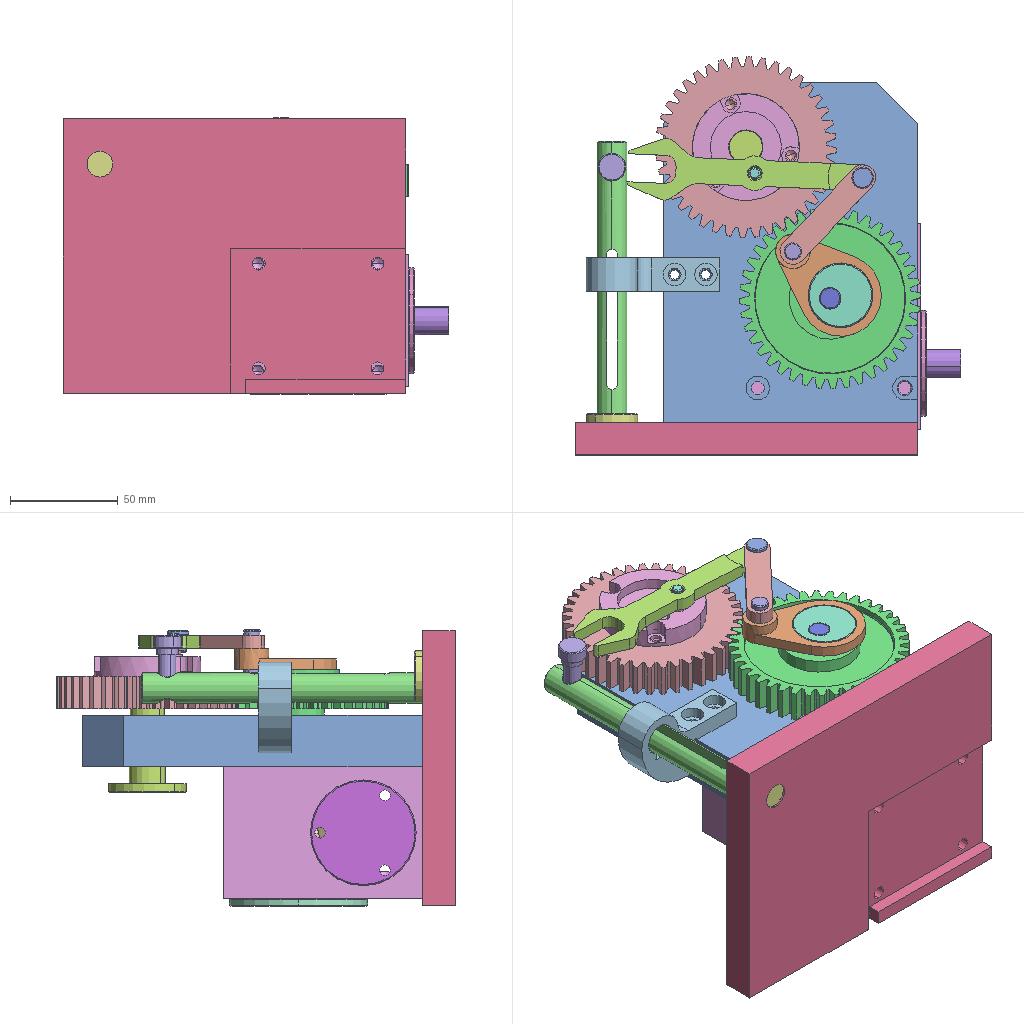Assembly | SolidWorks | 29 different items | 29 placed | box 178 x 184 x 128 mm
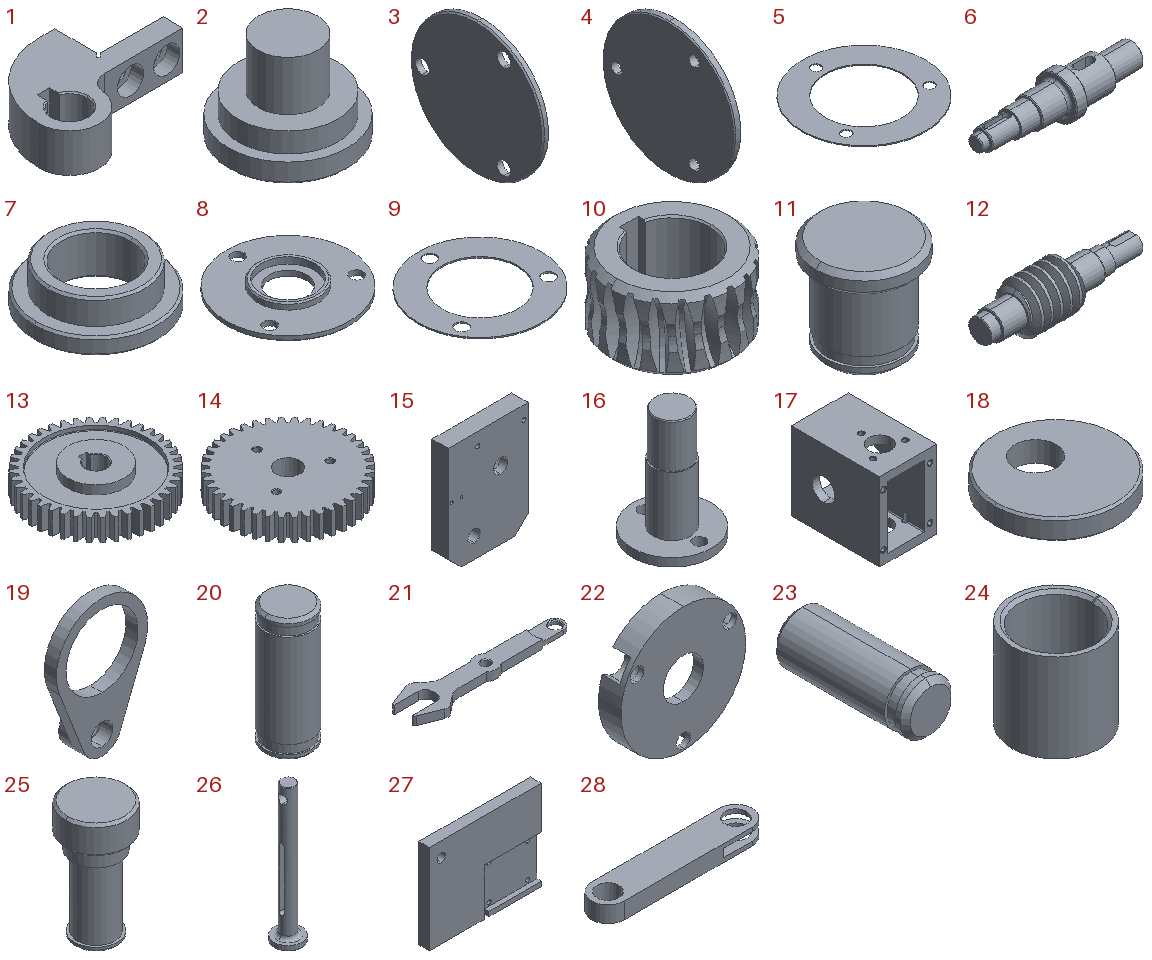Parts list (item | name | quantity | size | volume | features):
1 | - | x1 | 62 x 42 x 15.5 mm | 16029 mm3 | features ICE 3, Chamfer 1, Extrusion 1
2 | - | x1 | 24 x 24 x 18 mm | 4188 mm3 | features ICE 2, Chamfer 1, Extrusion 1
3 | - | x1 | 4.5 x 49 x 49 mm | 3890 mm3 | features ICE 3, Chamfer 1, Extrusion 1
4 | - | x1 | 6 x 64 x 64 mm | 11842 mm3 | features ICE 3, Chamfer 1, Extrusion 1
5 | - | x1 | 64 x 64 x 0.5 mm | 950.724 mm3 | features Extrusion 1, ICE 1
6 | - | x1 | 109 x 29 x 29 mm | 31302 mm3 | features ICE 8, Chamfer 1, Extrusion 1, Fillet 1
7 | - | x1 | 30 x 30 x 10 mm | 3114 mm3 | features Chamfer 2, ICE 2, Extrusion 1
8 | - | x1 | 49 x 49 x 4.5 mm | 3537 mm3 | features ICE 4, Chamfer 1, Extrusion 1
9 | - | x1 | 49 x 49 x 0.5 mm | 559.989 mm3 | features Extrusion 1, ICE 1
10 | - | x1 | 39.446 x 39.446 x 23 mm | 13124 mm3 | features Chamfer 2, CirPattern 1, Helix 1, ICE 1, Revolution 1, SweepCut 1
11 | - | x1 | 10 x 10 x 10 mm | 542.514 mm3 | features ICE 3, Chamfer 1, Extrusion 1
12 | - | x1 | 100.5 x 30 x 30 mm | 31439 mm3 | features ICE 6, Chamfer 1, Extrusion 1, Helix 1, RevCut 1, SweepCut 1
13 | - | x1 | 83.67 x 83.67 x 21 mm | 68213 mm3 | features ICE 5, Chamfer 2, CirPattern 1, Extrusion 1
14 | - | x1 | 83.602 x 83.602 x 15 mm | 71569 mm3 | features CirPattern 1, Extrusion 1, HoleWzd 1, ICE 1
15 | - | x1 | 117.5 x 24 x 160.5 mm | 414919 mm3 | features ICE 4, Chamfer 2, Extrusion 1, HoleWzd 1
16 | - | x1 | 36 x 36 x 51 mm | 14019 mm3 | features ICE 3, Chamfer 1, Extrusion 1
17 | - | x1 | 61 x 95 x 84 mm | 198920 mm3 | features HoleWzd 4, ICE 4, Extrusion 1, Fillet 1, MirrorPattern 1
18 | - | x1 | 30 x 30 x 5 mm | 3118 mm3 | features Chamfer 1, Extrusion 1, ICE 1
19 | - | x1 | 38 x 10 x 57 mm | 4565 mm3 | features ICE 3, Extrusion 1
20 | - | x1 | 8 x 8 x 21 mm | 1031 mm3 | features ICE 2, Chamfer 1, Extrusion 1, MirrorPattern 1
21 | - | x1 | 114.951 x 28.607 x 6 mm | 7418 mm3 | features ICE 2, Chamfer 1, Extrusion 1, Fillet 1, MirrorPattern 1
22 | - | x1 | 49.5 x 12 x 49.5 mm | 11403 mm3 | features ICE 6, CirPattern 1, Extrusion 1, HoleWzd 1
23 | - | x1 | 5 x 13 x 5 mm | 247.859 mm3 | features ICE 2, Chamfer 1, Extrusion 1
24 | - | x1 | 6 x 6 x 6 mm | 50.895 mm3 | features Chamfer 1, Extrusion 1, ICE 1
25 | - | x1 | 13 x 13 x 25 mm | 1836 mm3 | features ICE 4, Chamfer 1, Extrusion 1
26 | - | x1 | 28 x 28 x 140 mm | 18757 mm3 | features Chamfer 3, ICE 3, Extrusion 1, Fillet 1
27 | - | x1 | 158.5 x 15 x 127 mm | 237591 mm3 | features ICE 6, Extrusion 1, HoleWzd 1
28 | - | x1 | 59 x 12 x 6 mm | 3063 mm3 | features ICE 2, Extrusion 1
29 | angular contact ball bearings gb | x1 | - | - | -
Mates (type | each side: item.copy, entity, surface, feature):
Coincident | 27.1 plane | assembly plane | 3 times
Coincident | 27.1 face plane Cut-Extrude1 | 15.1 face plane Boss-Extrude1 | 3 times
Concentric | 14.1 face cylinder Boss-Extrude1 | 15.1 face cylinder Cut-Extrude1
Concentric | 15.1 face cylinder Cut-Extrude3 | 17.1 face cylinder Cut-Extrude3
Parallel | 15.1 face plane Boss-Extrude1 | 17.1 face plane Boss-Extrude1
Coincident | 15.1 face plane Boss-Extrude1 | 17.1 face plane Boss-Extrude1
Concentric | 13.1 face cylinder Cut-Extrude2 | 15.1 face cylinder Cut-Extrude3
Concentric | 12.1 face cylinder Boss-Extrude4 | 17.1 edge
Concentric | 10.1 face cylinder Revolve1 | 17.1 face cylinder Cut-Extrude3
Concentric | 18.1 face cylinder Boss-Extrude1 | 19.1 face cylinder Cut-Extrude1
Coincident | 18.1 face plane Boss-Extrude1 | 19.1 face plane Boss-Extrude1
Concentric | 6.1 face cylinder Boss-Extrude6 | 15.1 face cylinder Cut-Extrude1
Coincident | 6.1 face plane Cut-Extrude2 | 13.1 face plane Cut-Extrude2
Coincident | 6.1 face plane Boss-Extrude2 | 13.1 face plane Boss-Extrude3
Concentric | 6.1 face cylinder Boss-Extrude1 | 18.1 face cylinder Cut-Extrude1
Coincident | 6.1 face plane Boss-Extrude1 | 18.1 face plane Boss-Extrude1
Concentric | 15.1 face cylinder Cut-Extrude1 | 16.1 face cylinder Boss-Extrude2
Concentric | 28.1 face cylinder Cut-Extrude2 | 19.1 face cylinder Cut-Extrude1
Coincident | 28.1 face plane Boss-Extrude1 | 19.1 face plane Boss-Extrude2
Concentric | 28.1 face cylinder Cut-Extrude2 | 21.1 face cylinder Cut-Extrude2
Concentric | 11.1 face cylinder Boss-Extrude3 | 21.1 face cylinder Cut-Extrude2 | 2 times
Coincident | 28.1 face plane Boss-Extrude1 | 11.1 face plane Boss-Extrude4
Concentric | 1.1 face cylinder Cut-Extrude1 | 15.1 face cylinder M5 Tapped Hole1 | 2 times
Coincident | 1.1 face plane Boss-Extrude1 | 15.1 face plane Boss-Extrude1
Concentric | 26.1 face cylinder Boss-Extrude2 | 1.1 face cylinder Boss-Extrude1
Concentric | 25.1 face cylinder Boss-Extrude2 | 26.1 face cylinder Cut-Extrude2
Coincident | 28.1 face plane Cut-Extrude1 | 21.1 face plane Mirror1
Concentric | 19.1 face cylinder Cut-Extrude1 | 20.1 face cylinder Boss-Extrude1
Concentric | 21.1 edge | 23.1 face cylinder Boss-Extrude3
Coincident | 21.1 face plane Boss-Extrude1 | 23.1 edge
Coincident | 28.1 face plane Boss-Extrude1 | 20.1 face plane Boss-Extrude1
Concentric | 3.1 face cylinder Boss-Extrude2 | 17.1 face cylinder Mirror1
Concentric | 3.1 face cylinder Cut-Extrude2 | 17.1 face cylinder Mirror1
Coincident | 3.1 face plane Boss-Extrude1 | 17.1 face plane Boss-Extrude1
Concentric | 8.1 face cylinder Boss-Extrude2 | 17.1 face cylinder Cut-Extrude4
Concentric | 8.1 face cylinder Cut-Extrude3 | 17.1 face cylinder M6 Tapped Hole1
Concentric | 9.1 face cylinder Boss-Extrude1 | 12.1 face cylinder Boss-Extrude6
Coincident | 9.1 face plane Boss-Extrude1 | 17.1 face plane Boss-Extrude1
Concentric | 9.1 face cylinder Cut-Extrude1 | 17.1 face cylinder M6 Tapped Hole1
Coincident | 8.1 face plane Boss-Extrude1 | 9.1 face plane Boss-Extrude1
Concentric | 4.1 face cylinder Cut-Extrude1 | 17.1 face cylinder Cut-Extrude2
Concentric | 4.1 face cylinder Cut-Extrude2 | 17.1 edge
Concentric | 4.1 face cylinder Cut-Extrude1 | 5.1 face cylinder Boss-Extrude1
Concentric | 5.1 face cylinder Cut-Extrude1 | 17.1 face cylinder M5 Tapped Hole1
Coincident | 5.1 face plane Boss-Extrude1 | 17.1 face plane Boss-Extrude1
Coincident | 4.1 face plane Boss-Extrude1 | 5.1 face plane Boss-Extrude1
Coincident | 22.1 face plane Boss-Extrude1 | 14.1 face plane Boss-Extrude1
Tangent | 22.1 face cylinder CirPattern1 | 14.1 face cylinder M5 Tapped Hole1
Coincident | 13.1 face plane Boss-Extrude1 | 14.1 face plane Boss-Extrude1
Concentric | 22.1 face cylinder Cut-Extrude4 | 14.1 face cylinder Boss-Extrude1
Concentric | 22.1 face cylinder Ø5.0mm blind dowel hole 1 | 23.1 face cylinder Boss-Extrude2
Parallel | 21.1 face plane Boss-Extrude1 | 25.1 face plane Boss-Extrude5
Tangent | 21.1 face plane Boss-Extrude1 | 25.1 face cylinder Boss-Extrude5
Coincident | 21.1 face plane Boss-Extrude1 | 25.1 face plane Boss-Extrude5
Concentric | 6.1 face cylinder Boss-Extrude7 | 7.1 face cylinder Cut-Extrude1
Coincident | 7.1 face plane Boss-Extrude1 | 10.1 face plane Revolve1
Coincident | 7.1 face plane Boss-Extrude2 | 17.1 face plane Cut-Extrude1
Concentric | 27.1 face cylinder Cut-Extrude6 | 2.1 face cylinder Boss-Extrude1
Coincident | 27.1 face plane Boss-Extrude1 | 2.1 face plane Boss-Extrude3
Concentric | 23.1 face cylinder Boss-Extrude3 | 24.1 face cylinder Boss-Extrude1
Coincident | 23.1 face plane Boss-Extrude3 | 24.1 face plane Boss-Extrude1
GearDim | 14.1 edge | 13.1 edge
Coincident | 12.1 edge | 17.1 face plane Cut-Extrude1